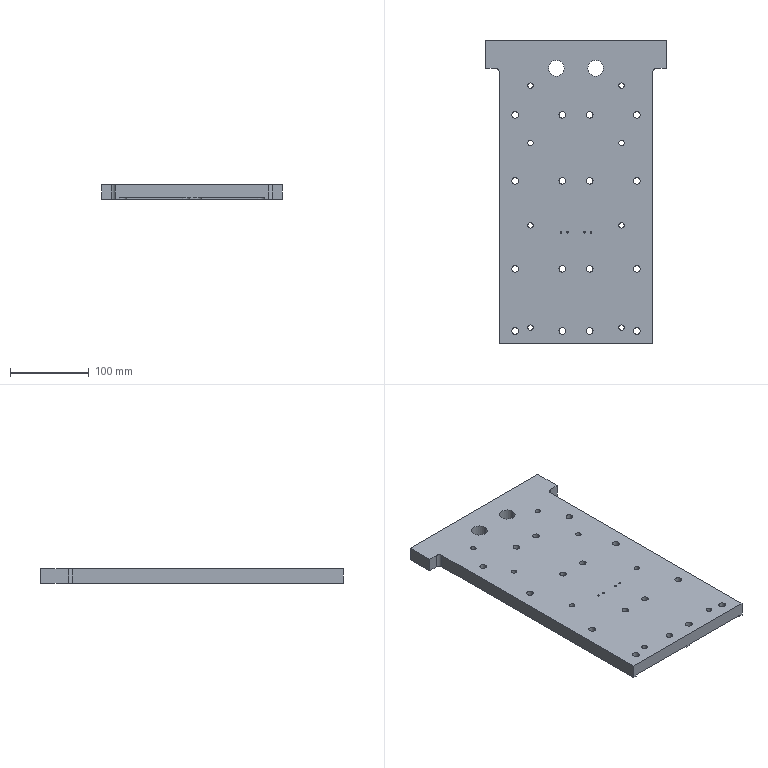NC program | NX | posted with a generic post | part box 230 x 385 x 18 mm
Lines 1 to 83 of 3056:
N10 G17 G21 G94 G90
(DRILLING , TOOL : D6A45)
N12 T01 M6
N14 G54
N16 G17 G0 G90 X98.2 Y-17.5 S5000 M3
N18 G43 Z30. H1
N20 G94 G81 G98 Z-1. F350. R3.
N22 Y17.5
N24 X62.5 Y58.
N26 X98.2 Y77.5
N28 X135.5 Y58.
N30 X157.5 Y25.
N32 Y-25.
N34 X135.5 Y-58.
N36 X98.2 Y-77.5
N38 X62.5 Y-58.
N40 X14.2 Y-77.5
N42 Y-17.5
N44 Y17.5
N46 Y77.5
N48 X-42.5 Y58.
N50 X-97.8 Y77.5
N52 Y17.5
N54 Y-17.5
N56 X-42.5 Y-58.
N58 X-97.8 Y-77.5
N60 X-176.8
N62 X-172.5 Y-58.
N64 X-176.8 Y-17.5
N66 Y17.5
N68 X-172.5 Y58.
N70 X-176.8 Y77.5
N72 G80
N74 G0 X-176.8 Y77.5 Z30.
N76 M5
(DRILLING_COPY_COPY_COPY , TOOL : 6.8ZT)
N78 T06 M6
N80 G54
N82 G17 G0 G90 X-42.5 Y-58. S2000 M3
N84 G43 Z30. H6
N86 G94 G83 G98 Z-21.043 F300. Q2. R3.
N88 X62.5
N90 X135.5
N92 Y58.
N94 X62.5
N96 X-42.5
N98 X-172.5
N100 Y-58.
N102 G80
N104 G0 X-172.5 Y-58. Z30.
N106 M5
(DRILLING_COPY_COPY_COPY_COPY , TOOL : 8.5ZT)
N108 T16 M6
N110 G54
N112 G17 G0 G90 X98.2 Y77.5 S2000 M3
N114 G43 Z30. H16
N116 G94 G83 G98 Z-21.554 F300. Q2. R3.
N118 Y17.5
N120 Y-17.5
N122 Y-77.5
N124 X14.2
N126 Y-17.5
N128 Y17.5
N130 Y77.5
N132 X-97.8
N134 Y17.5
N136 Y-17.5
N138 Y-77.5
N140 X-176.8
N142 Y-17.5
N144 Y17.5
N146 Y77.5
N148 G80
N150 G0 X-176.8 Y77.5 Z30.
N152 M5